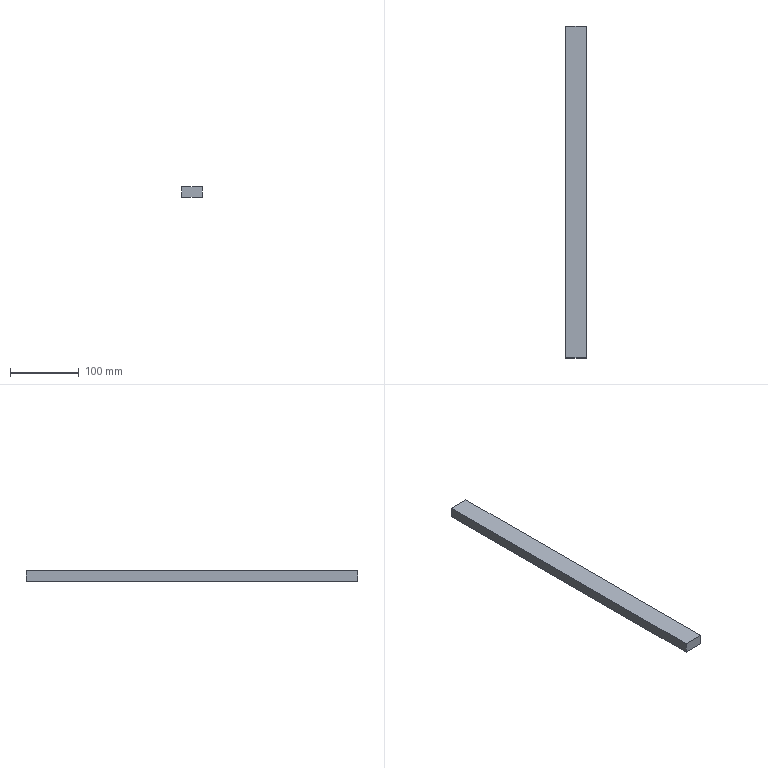Part | NX | features solid 2 | 1 solid | 6 faces | box 30 x 482.5 x 15 mm | volume 217125 mm3 | plane 6
STEP:
#1=CARTESIAN_POINT('',(465.,-482.5,-69.));
#2=VERTEX_POINT('',#1);
#3=CARTESIAN_POINT('',(495.,-482.5,-69.));
#4=VERTEX_POINT('',#3);
#5=CARTESIAN_POINT('',(615.,-482.5,-69.));
#6=DIRECTION('',(1.,0.,0.));
#7=VECTOR('',#6,1000.);
#8=LINE('',#5,#7);
#9=EDGE_CURVE('',#2,#4,#8,.T.);
#10=ORIENTED_EDGE('',*,*,#9,.F.);
#11=CARTESIAN_POINT('',(465.,-482.5,-84.));
#12=VERTEX_POINT('',#11);
#13=CARTESIAN_POINT('',(465.,-482.5,-84.));
#14=DIRECTION('',(0.,0.,-1.));
#15=VECTOR('',#14,1000.);
#16=LINE('',#13,#15);
#17=EDGE_CURVE('',#12,#2,#16,.F.);
#18=ORIENTED_EDGE('',*,*,#17,.F.);
#19=CARTESIAN_POINT('',(495.,-482.5,-84.));
#20=VERTEX_POINT('',#19);
#21=CARTESIAN_POINT('',(615.,-482.5,-84.));
#22=DIRECTION('',(-1.,0.,0.));
#23=VECTOR('',#22,1000.);
#24=LINE('',#21,#23);
#25=EDGE_CURVE('',#12,#20,#24,.F.);
#26=ORIENTED_EDGE('',*,*,#25,.T.);
#27=CARTESIAN_POINT('',(495.,-482.5,-84.));
#28=DIRECTION('',(0.,0.,-1.));
#29=VECTOR('',#28,1000.);
#30=LINE('',#27,#29);
#31=EDGE_CURVE('',#20,#4,#30,.F.);
#32=ORIENTED_EDGE('',*,*,#31,.T.);
#33=EDGE_LOOP('',(#10,#18,#26,#32));
#34=FACE_BOUND('',#33,.T.);
#35=CARTESIAN_POINT('',(615.,-482.5,-84.));
#36=DIRECTION('',(0.,-1.,0.));
#37=DIRECTION('',(0.,0.,1.));
#38=AXIS2_PLACEMENT_3D('',#35,#36,#37);
#39=PLANE('',#38);
#40=ADVANCED_FACE('',(#34),#39,.T.);
#41=ORIENTED_EDGE('',*,*,#25,.F.);
#42=CARTESIAN_POINT('',(465.,0.,-84.));
#43=VERTEX_POINT('',#42);
#44=CARTESIAN_POINT('',(465.,-462.5,-84.));
#45=DIRECTION('',(0.,1.,0.));
#46=VECTOR('',#45,1000.);
#47=LINE('',#44,#46);
#48=EDGE_CURVE('',#12,#43,#47,.T.);
#49=ORIENTED_EDGE('',*,*,#48,.T.);
#50=CARTESIAN_POINT('',(495.,0.,-84.));
#51=VERTEX_POINT('',#50);
#52=CARTESIAN_POINT('',(615.,0.,-84.));
#53=DIRECTION('',(1.,0.,0.));
#54=VECTOR('',#53,1000.);
#55=LINE('',#52,#54);
#56=EDGE_CURVE('',#43,#51,#55,.T.);
#57=ORIENTED_EDGE('',*,*,#56,.T.);
#58=CARTESIAN_POINT('',(495.,-462.5,-84.));
#59=DIRECTION('',(0.,1.,0.));
#60=VECTOR('',#59,1000.);
#61=LINE('',#58,#60);
#62=EDGE_CURVE('',#20,#51,#61,.T.);
#63=ORIENTED_EDGE('',*,*,#62,.F.);
#64=EDGE_LOOP('',(#41,#49,#57,#63));
#65=FACE_BOUND('',#64,.T.);
#66=CARTESIAN_POINT('',(615.,-462.5,-84.));
#67=DIRECTION('',(0.,0.,1.));
#68=DIRECTION('',(0.,1.,0.));
#69=AXIS2_PLACEMENT_3D('',#66,#67,#68);
#70=PLANE('',#69);
#71=ADVANCED_FACE('',(#65),#70,.F.);
#72=ORIENTED_EDGE('',*,*,#56,.F.);
#73=CARTESIAN_POINT('',(465.,0.,-69.));
#74=VERTEX_POINT('',#73);
#75=CARTESIAN_POINT('',(465.,0.,-69.));
#76=DIRECTION('',(0.,0.,1.));
#77=VECTOR('',#76,1000.);
#78=LINE('',#75,#77);
#79=EDGE_CURVE('',#43,#74,#78,.T.);
#80=ORIENTED_EDGE('',*,*,#79,.T.);
#81=CARTESIAN_POINT('',(495.,0.,-69.));
#82=VERTEX_POINT('',#81);
#83=CARTESIAN_POINT('',(542.5,0.,-69.));
#84=DIRECTION('',(-1.,0.,0.));
#85=VECTOR('',#84,1000.);
#86=LINE('',#83,#85);
#87=EDGE_CURVE('',#74,#82,#86,.F.);
#88=ORIENTED_EDGE('',*,*,#87,.T.);
#89=CARTESIAN_POINT('',(495.,0.,-69.));
#90=DIRECTION('',(0.,0.,1.));
#91=VECTOR('',#90,1000.);
#92=LINE('',#89,#91);
#93=EDGE_CURVE('',#51,#82,#92,.T.);
#94=ORIENTED_EDGE('',*,*,#93,.F.);
#95=EDGE_LOOP('',(#72,#80,#88,#94));
#96=FACE_BOUND('',#95,.T.);
#97=CARTESIAN_POINT('',(542.5,0.,-69.));
#98=DIRECTION('',(0.,-1.,0.));
#99=DIRECTION('',(0.,0.,-1.));
#100=AXIS2_PLACEMENT_3D('',#97,#98,#99);
#101=PLANE('',#100);
#102=ADVANCED_FACE('',(#96),#101,.F.);
#103=CARTESIAN_POINT('',(465.,-462.5,-69.));
#104=DIRECTION('',(0.,-1.,0.));
#105=VECTOR('',#104,1000.);
#106=LINE('',#103,#105);
#107=EDGE_CURVE('',#2,#74,#106,.F.);
#108=ORIENTED_EDGE('',*,*,#107,.F.);
#109=ORIENTED_EDGE('',*,*,#9,.T.);
#110=CARTESIAN_POINT('',(495.,-462.5,-69.));
#111=DIRECTION('',(0.,-1.,0.));
#112=VECTOR('',#111,1000.);
#113=LINE('',#110,#112);
#114=EDGE_CURVE('',#4,#82,#113,.F.);
#115=ORIENTED_EDGE('',*,*,#114,.T.);
#116=ORIENTED_EDGE('',*,*,#87,.F.);
#117=EDGE_LOOP('',(#108,#109,#115,#116));
#118=FACE_BOUND('',#117,.T.);
#119=CARTESIAN_POINT('',(615.,-462.5,-69.));
#120=DIRECTION('',(0.,0.,1.));
#121=DIRECTION('',(0.,1.,0.));
#122=AXIS2_PLACEMENT_3D('',#119,#120,#121);
#123=PLANE('',#122);
#124=ADVANCED_FACE('',(#118),#123,.T.);
#125=ORIENTED_EDGE('',*,*,#93,.T.);
#126=ORIENTED_EDGE('',*,*,#114,.F.);
#127=ORIENTED_EDGE('',*,*,#31,.F.);
#128=ORIENTED_EDGE('',*,*,#62,.T.);
#129=EDGE_LOOP('',(#125,#126,#127,#128));
#130=FACE_BOUND('',#129,.T.);
#131=CARTESIAN_POINT('',(495.,-462.5,-84.));
#132=DIRECTION('',(1.,0.,0.));
#133=DIRECTION('',(0.,0.,-1.));
#134=AXIS2_PLACEMENT_3D('',#131,#132,#133);
#135=PLANE('',#134);
#136=ADVANCED_FACE('',(#130),#135,.T.);
#137=ORIENTED_EDGE('',*,*,#79,.F.);
#138=ORIENTED_EDGE('',*,*,#48,.F.);
#139=ORIENTED_EDGE('',*,*,#17,.T.);
#140=ORIENTED_EDGE('',*,*,#107,.T.);
#141=EDGE_LOOP('',(#137,#138,#139,#140));
#142=FACE_BOUND('',#141,.T.);
#143=CARTESIAN_POINT('',(465.,-462.5,-84.));
#144=DIRECTION('',(1.,0.,0.));
#145=DIRECTION('',(0.,0.,-1.));
#146=AXIS2_PLACEMENT_3D('',#143,#144,#145);
#147=PLANE('',#146);
#148=ADVANCED_FACE('',(#142),#147,.F.);
#149=CLOSED_SHELL('',(#40,#71,#102,#124,#136,#148));
#150=MANIFOLD_SOLID_BREP('',#149);
#151=(LENGTH_UNIT()NAMED_UNIT(*)SI_UNIT(.MILLI.,.METRE.));
#152=UNCERTAINTY_MEASURE_WITH_UNIT(LENGTH_MEASURE(0.00001),#151,'','');
#153=(NAMED_UNIT(*)PLANE_ANGLE_UNIT()SI_UNIT($,.RADIAN.));
#154=(NAMED_UNIT(*)SI_UNIT($,.STERADIAN.)SOLID_ANGLE_UNIT());
#155=(GEOMETRIC_REPRESENTATION_CONTEXT(3)GLOBAL_UNCERTAINTY_ASSIGNED_CONTEXT((#152))GLOBAL_UNIT_ASSIGNED_CONTEXT((#151,#153,#154))REPRESENTATION_CONTEXT('',''));
#156=ADVANCED_BREP_SHAPE_REPRESENTATION('',(#150),#155);